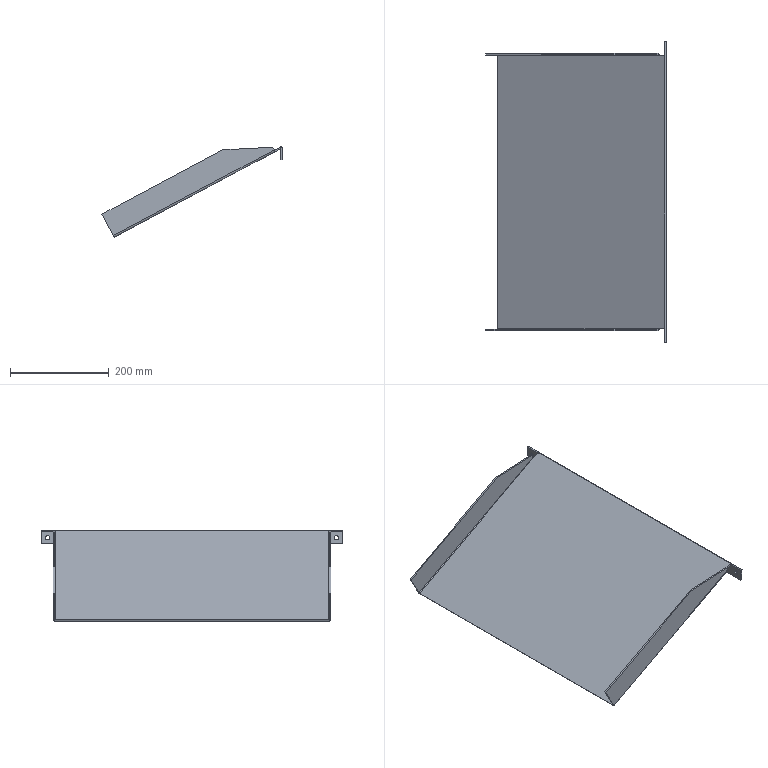Part | STEP file | lll_id3818_x_t | 1 solid | 27 faces | box 365.363 x 612 x 183.438 mm | volume 789228 mm3 | plane 20 | cylinder 7 | commonest cylinder face diameters 2 x2 8 x2 9 x2 3 x1
STEP:
#1=CARTESIAN_POINT('',(3904.435,-293.,-189.665));
#2=VERTEX_POINT('',#1);
#3=CARTESIAN_POINT('',(3904.435,-293.,-194.165));
#4=DIRECTION('',(1.,0.,0.));
#5=DIRECTION('',(0.,0.,1.));
#6=AXIS2_PLACEMENT_3D('',#3,#4,#5);
#7=CIRCLE('',#6,4.5);
#8=EDGE_CURVE('',#2,#2,#7,.T.);
#9=ORIENTED_EDGE('',*,*,#8,.T.);
#10=EDGE_LOOP('',(#9));
#11=FACE_BOUND('',#10,.T.);
#12=CARTESIAN_POINT('',(3904.435,293.,-189.665));
#13=VERTEX_POINT('',#12);
#14=CARTESIAN_POINT('',(3904.435,293.,-194.165));
#15=DIRECTION('',(1.,0.,0.));
#16=DIRECTION('',(0.,0.,1.));
#17=AXIS2_PLACEMENT_3D('',#14,#15,#16);
#18=CIRCLE('',#17,4.5);
#19=EDGE_CURVE('',#13,#13,#18,.T.);
#20=ORIENTED_EDGE('',*,*,#19,.T.);
#21=EDGE_LOOP('',(#20));
#22=FACE_BOUND('',#21,.T.);
#23=CARTESIAN_POINT('',(3904.435,276.,-181.5));
#24=VERTEX_POINT('',#23);
#25=CARTESIAN_POINT('',(3904.435,276.,-183.996));
#26=VERTEX_POINT('',#25);
#27=CARTESIAN_POINT('',(3904.435,276.,-170.446));
#28=DIRECTION('',(0.,0.,-1.));
#29=VECTOR('',#28,1.);
#30=LINE('',#27,#29);
#31=EDGE_CURVE('',#24,#26,#30,.T.);
#32=ORIENTED_EDGE('',*,*,#31,.F.);
#33=CARTESIAN_POINT('',(3904.435,306.,-181.5));
#34=VERTEX_POINT('',#33);
#35=CARTESIAN_POINT('',(3904.435,0.,-181.5));
#36=DIRECTION('',(0.,-1.,0.));
#37=VECTOR('',#36,1.);
#38=LINE('',#35,#37);
#39=EDGE_CURVE('',#34,#24,#38,.T.);
#40=ORIENTED_EDGE('',*,*,#39,.F.);
#41=CARTESIAN_POINT('',(3904.435,306.,-206.165));
#42=VERTEX_POINT('',#41);
#43=CARTESIAN_POINT('',(3904.435,306.,-170.446));
#44=DIRECTION('',(0.,0.,-1.));
#45=VECTOR('',#44,1.);
#46=LINE('',#43,#45);
#47=EDGE_CURVE('',#34,#42,#46,.T.);
#48=ORIENTED_EDGE('',*,*,#47,.T.);
#49=CARTESIAN_POINT('',(3904.435,-306.,-206.165));
#50=VERTEX_POINT('',#49);
#51=CARTESIAN_POINT('',(3904.435,110.,-206.165));
#52=DIRECTION('',(0.,-1.,0.));
#53=VECTOR('',#52,1.);
#54=LINE('',#51,#53);
#55=EDGE_CURVE('',#42,#50,#54,.T.);
#56=ORIENTED_EDGE('',*,*,#55,.T.);
#57=CARTESIAN_POINT('',(3904.435,-306.,-181.5));
#58=VERTEX_POINT('',#57);
#59=CARTESIAN_POINT('',(3904.435,-306.,-170.446));
#60=DIRECTION('',(0.,0.,1.));
#61=VECTOR('',#60,1.);
#62=LINE('',#59,#61);
#63=EDGE_CURVE('',#50,#58,#62,.T.);
#64=ORIENTED_EDGE('',*,*,#63,.T.);
#65=CARTESIAN_POINT('',(3904.435,-276.,-181.5));
#66=VERTEX_POINT('',#65);
#67=CARTESIAN_POINT('',(3904.435,0.,-181.5));
#68=DIRECTION('',(0.,-1.,0.));
#69=VECTOR('',#68,1.);
#70=LINE('',#67,#69);
#71=EDGE_CURVE('',#66,#58,#70,.T.);
#72=ORIENTED_EDGE('',*,*,#71,.F.);
#73=CARTESIAN_POINT('',(3904.435,-276.,-183.996));
#74=VERTEX_POINT('',#73);
#75=CARTESIAN_POINT('',(3904.435,-276.,-170.446));
#76=DIRECTION('',(0.,0.,1.));
#77=VECTOR('',#76,1.);
#78=LINE('',#75,#77);
#79=EDGE_CURVE('',#74,#66,#78,.T.);
#80=ORIENTED_EDGE('',*,*,#79,.F.);
#81=CARTESIAN_POINT('',(3904.435,110.,-183.996));
#82=DIRECTION('',(0.,-1.,0.));
#83=VECTOR('',#82,1.);
#84=LINE('',#81,#83);
#85=EDGE_CURVE('',#26,#74,#84,.T.);
#86=ORIENTED_EDGE('',*,*,#85,.F.);
#87=EDGE_LOOP('',(#32,#40,#48,#56,#64,#72,#80,#86));
#88=FACE_BOUND('',#87,.T.);
#89=CARTESIAN_POINT('',(3904.435,110.,-170.446));
#90=DIRECTION('',(1.,0.,0.));
#91=DIRECTION('',(0.,0.,-1.));
#92=AXIS2_PLACEMENT_3D('',#89,#90,#91);
#93=PLANE('',#92);
#94=ADVANCED_FACE('',(#11,#22,#88),#93,.F.);
#95=CARTESIAN_POINT('',(3907.435,-306.,-206.165));
#96=VERTEX_POINT('',#95);
#97=CARTESIAN_POINT('',(3907.435,-306.,-181.5));
#98=VERTEX_POINT('',#97);
#99=CARTESIAN_POINT('',(3907.435,-306.,-170.446));
#100=DIRECTION('',(0.,0.,1.));
#101=VECTOR('',#100,1.);
#102=LINE('',#99,#101);
#103=EDGE_CURVE('',#96,#98,#102,.T.);
#104=ORIENTED_EDGE('',*,*,#103,.F.);
#105=CARTESIAN_POINT('',(3907.435,306.,-206.165));
#106=VERTEX_POINT('',#105);
#107=CARTESIAN_POINT('',(3907.435,285.,-206.165));
#108=DIRECTION('',(0.,-1.,0.));
#109=VECTOR('',#108,1.);
#110=LINE('',#107,#109);
#111=EDGE_CURVE('',#106,#96,#110,.T.);
#112=ORIENTED_EDGE('',*,*,#111,.F.);
#113=CARTESIAN_POINT('',(3907.435,306.,-181.5));
#114=VERTEX_POINT('',#113);
#115=CARTESIAN_POINT('',(3907.435,306.,-170.446));
#116=DIRECTION('',(0.,0.,-1.));
#117=VECTOR('',#116,1.);
#118=LINE('',#115,#117);
#119=EDGE_CURVE('',#114,#106,#118,.T.);
#120=ORIENTED_EDGE('',*,*,#119,.F.);
#121=CARTESIAN_POINT('',(3907.435,36.,-181.5));
#122=DIRECTION('',(0.,1.,0.));
#123=VECTOR('',#122,1.);
#124=LINE('',#121,#123);
#125=EDGE_CURVE('',#98,#114,#124,.T.);
#126=ORIENTED_EDGE('',*,*,#125,.F.);
#127=EDGE_LOOP('',(#104,#112,#120,#126));
#128=FACE_BOUND('',#127,.T.);
#129=CARTESIAN_POINT('',(3907.435,293.,-198.665));
#130=VERTEX_POINT('',#129);
#131=CARTESIAN_POINT('',(3907.435,293.,-194.165));
#132=DIRECTION('',(1.,0.,0.));
#133=DIRECTION('',(0.,0.,-1.));
#134=AXIS2_PLACEMENT_3D('',#131,#132,#133);
#135=CIRCLE('',#134,4.5);
#136=EDGE_CURVE('',#130,#130,#135,.T.);
#137=ORIENTED_EDGE('',*,*,#136,.F.);
#138=EDGE_LOOP('',(#137));
#139=FACE_BOUND('',#138,.T.);
#140=CARTESIAN_POINT('',(3907.435,-293.,-198.665));
#141=VERTEX_POINT('',#140);
#142=CARTESIAN_POINT('',(3907.435,-293.,-194.165));
#143=DIRECTION('',(1.,0.,0.));
#144=DIRECTION('',(0.,0.,-1.));
#145=AXIS2_PLACEMENT_3D('',#142,#143,#144);
#146=CIRCLE('',#145,4.5);
#147=EDGE_CURVE('',#141,#141,#146,.T.);
#148=ORIENTED_EDGE('',*,*,#147,.F.);
#149=EDGE_LOOP('',(#148));
#150=FACE_BOUND('',#149,.T.);
#151=CARTESIAN_POINT('',(3907.435,110.,-170.446));
#152=DIRECTION('',(1.,0.,0.));
#153=DIRECTION('',(0.,0.,-1.));
#154=AXIS2_PLACEMENT_3D('',#151,#152,#153);
#155=PLANE('',#154);
#156=ADVANCED_FACE('',(#128,#139,#150),#155,.T.);
#157=ORIENTED_EDGE('',*,*,#103,.T.);
#158=CARTESIAN_POINT('',(3905.935,-306.,-181.5));
#159=DIRECTION('',(0.,1.,0.));
#160=DIRECTION('',(0.,0.,1.));
#161=AXIS2_PLACEMENT_3D('',#158,#159,#160);
#162=CIRCLE('',#161,1.5);
#163=EDGE_CURVE('',#58,#98,#162,.T.);
#164=ORIENTED_EDGE('',*,*,#163,.F.);
#165=ORIENTED_EDGE('',*,*,#63,.F.);
#166=CARTESIAN_POINT('',(3907.435,-306.,-206.165));
#167=DIRECTION('',(1.,0.,0.));
#168=VECTOR('',#167,1.);
#169=LINE('',#166,#168);
#170=EDGE_CURVE('',#50,#96,#169,.T.);
#171=ORIENTED_EDGE('',*,*,#170,.T.);
#172=EDGE_LOOP('',(#157,#164,#165,#171));
#173=FACE_OUTER_BOUND('',#172,.T.);
#174=CARTESIAN_POINT('',(3907.435,-306.,-173.053));
#175=DIRECTION('',(0.,1.,0.));
#176=DIRECTION('',(0.,0.,-1.));
#177=AXIS2_PLACEMENT_3D('',#174,#175,#176);
#178=PLANE('',#177);
#179=ADVANCED_FACE('',(#173),#178,.F.);
#180=ORIENTED_EDGE('',*,*,#170,.F.);
#181=ORIENTED_EDGE('',*,*,#55,.F.);
#182=CARTESIAN_POINT('',(3907.435,306.,-206.165));
#183=DIRECTION('',(1.,0.,0.));
#184=VECTOR('',#183,1.);
#185=LINE('',#182,#184);
#186=EDGE_CURVE('',#42,#106,#185,.T.);
#187=ORIENTED_EDGE('',*,*,#186,.T.);
#188=ORIENTED_EDGE('',*,*,#111,.T.);
#189=EDGE_LOOP('',(#180,#181,#187,#188));
#190=FACE_OUTER_BOUND('',#189,.T.);
#191=CARTESIAN_POINT('',(3907.435,285.,-206.165));
#192=DIRECTION('',(0.,0.,-1.));
#193=DIRECTION('',(0.,-1.,0.));
#194=AXIS2_PLACEMENT_3D('',#191,#192,#193);
#195=PLANE('',#194);
#196=ADVANCED_FACE('',(#190),#195,.T.);
#197=ORIENTED_EDGE('',*,*,#47,.F.);
#198=CARTESIAN_POINT('',(3905.935,306.,-181.5));
#199=DIRECTION('',(0.,-1.,0.));
#200=DIRECTION('',(1.,0.,0.));
#201=AXIS2_PLACEMENT_3D('',#198,#199,#200);
#202=CIRCLE('',#201,1.5);
#203=EDGE_CURVE('',#114,#34,#202,.T.);
#204=ORIENTED_EDGE('',*,*,#203,.F.);
#205=ORIENTED_EDGE('',*,*,#119,.T.);
#206=ORIENTED_EDGE('',*,*,#186,.F.);
#207=EDGE_LOOP('',(#197,#204,#205,#206));
#208=FACE_OUTER_BOUND('',#207,.T.);
#209=CARTESIAN_POINT('',(3887.906,306.,-180.316));
#210=DIRECTION('',(0.,-1.,0.));
#211=DIRECTION('',(-0.5,0.,0.866));
#212=AXIS2_PLACEMENT_3D('',#209,#210,#211);
#213=PLANE('',#212);
#214=ADVANCED_FACE('',(#208),#213,.F.);
#215=CARTESIAN_POINT('',(3891.925,276.,-187.25));
#216=VERTEX_POINT('',#215);
#217=CARTESIAN_POINT('',(3905.231,276.,-180.176));
#218=VERTEX_POINT('',#217);
#219=CARTESIAN_POINT('',(3906.063,276.,-179.733));
#220=DIRECTION('',(0.8829,0.,0.4695));
#221=VECTOR('',#220,1.);
#222=LINE('',#219,#221);
#223=EDGE_CURVE('',#216,#218,#222,.T.);
#224=ORIENTED_EDGE('',*,*,#223,.F.);
#225=CARTESIAN_POINT('',(3891.925,277.,-187.25));
#226=VERTEX_POINT('',#225);
#227=CARTESIAN_POINT('',(3891.925,-109.,-187.25));
#228=DIRECTION('',(0.,-1.,0.));
#229=VECTOR('',#228,1.);
#230=LINE('',#227,#229);
#231=EDGE_CURVE('',#226,#216,#230,.T.);
#232=ORIENTED_EDGE('',*,*,#231,.F.);
#233=CARTESIAN_POINT('',(3565.546,277.,-360.789));
#234=VERTEX_POINT('',#233);
#235=CARTESIAN_POINT('',(3985.528,277.,-137.481));
#236=DIRECTION('',(0.8829,0.,0.4695));
#237=VECTOR('',#236,1.);
#238=LINE('',#235,#237);
#239=EDGE_CURVE('',#234,#226,#238,.T.);
#240=ORIENTED_EDGE('',*,*,#239,.F.);
#241=CARTESIAN_POINT('',(3565.546,-277.,-360.789));
#242=VERTEX_POINT('',#241);
#243=CARTESIAN_POINT('',(3565.546,-35.,-360.789));
#244=DIRECTION('',(0.,1.,0.));
#245=VECTOR('',#244,1.);
#246=LINE('',#243,#245);
#247=EDGE_CURVE('',#242,#234,#246,.T.);
#248=ORIENTED_EDGE('',*,*,#247,.F.);
#249=CARTESIAN_POINT('',(3891.925,-277.,-187.25));
#250=VERTEX_POINT('',#249);
#251=CARTESIAN_POINT('',(3985.528,-277.,-137.481));
#252=DIRECTION('',(-0.8829,0.,-0.4695));
#253=VECTOR('',#252,1.);
#254=LINE('',#251,#253);
#255=EDGE_CURVE('',#250,#242,#254,.T.);
#256=ORIENTED_EDGE('',*,*,#255,.F.);
#257=CARTESIAN_POINT('',(3891.925,-276.,-187.25));
#258=VERTEX_POINT('',#257);
#259=CARTESIAN_POINT('',(3891.925,2.,-187.25));
#260=DIRECTION('',(0.,-1.,0.));
#261=VECTOR('',#260,1.);
#262=LINE('',#259,#261);
#263=EDGE_CURVE('',#258,#250,#262,.T.);
#264=ORIENTED_EDGE('',*,*,#263,.F.);
#265=CARTESIAN_POINT('',(3905.231,-276.,-180.176));
#266=VERTEX_POINT('',#265);
#267=CARTESIAN_POINT('',(3906.063,-276.,-179.733));
#268=DIRECTION('',(-0.8829,0.,-0.4695));
#269=VECTOR('',#268,1.);
#270=LINE('',#267,#269);
#271=EDGE_CURVE('',#266,#258,#270,.T.);
#272=ORIENTED_EDGE('',*,*,#271,.F.);
#273=CARTESIAN_POINT('',(3905.231,0.,-180.176));
#274=DIRECTION('',(0.,-1.,0.));
#275=VECTOR('',#274,1.);
#276=LINE('',#273,#275);
#277=EDGE_CURVE('',#218,#266,#276,.T.);
#278=ORIENTED_EDGE('',*,*,#277,.F.);
#279=EDGE_LOOP('',(#224,#232,#240,#248,#256,#264,#272,#278));
#280=FACE_OUTER_BOUND('',#279,.T.);
#281=CARTESIAN_POINT('',(3906.063,-35.,-179.733));
#282=DIRECTION('',(-0.4695,0.,0.8829));
#283=DIRECTION('',(-0.8829,0.,-0.4695));
#284=AXIS2_PLACEMENT_3D('',#281,#282,#283);
#285=PLANE('',#284);
#286=ADVANCED_FACE('',(#280),#285,.T.);
#287=CARTESIAN_POINT('',(3893.333,276.,-189.899));
#288=VERTEX_POINT('',#287);
#289=CARTESIAN_POINT('',(3891.925,276.,-187.25));
#290=DIRECTION('',(-0.4695,0.,0.8829));
#291=VECTOR('',#290,1.);
#292=LINE('',#289,#291);
#293=EDGE_CURVE('',#288,#216,#292,.T.);
#294=ORIENTED_EDGE('',*,*,#293,.T.);
#295=ORIENTED_EDGE('',*,*,#223,.T.);
#296=CARTESIAN_POINT('',(3905.935,276.,-181.5));
#297=DIRECTION('',(0.,1.,0.));
#298=DIRECTION('',(0.,0.,-1.));
#299=AXIS2_PLACEMENT_3D('',#296,#297,#298);
#300=CIRCLE('',#299,1.5);
#301=EDGE_CURVE('',#24,#218,#300,.T.);
#302=ORIENTED_EDGE('',*,*,#301,.F.);
#303=ORIENTED_EDGE('',*,*,#31,.T.);
#304=CARTESIAN_POINT('',(3907.471,276.,-182.382));
#305=DIRECTION('',(0.8829,0.,0.4695));
#306=VECTOR('',#305,1.);
#307=LINE('',#304,#306);
#308=EDGE_CURVE('',#288,#26,#307,.T.);
#309=ORIENTED_EDGE('',*,*,#308,.F.);
#310=EDGE_LOOP('',(#294,#295,#302,#303,#309));
#311=FACE_OUTER_BOUND('',#310,.T.);
#312=CARTESIAN_POINT('',(3906.155,276.,-179.742));
#313=DIRECTION('',(0.,-1.,0.));
#314=DIRECTION('',(-0.9063,0.,-0.4226));
#315=AXIS2_PLACEMENT_3D('',#312,#313,#314);
#316=PLANE('',#315);
#317=ADVANCED_FACE('',(#311),#316,.F.);
#318=ORIENTED_EDGE('',*,*,#271,.T.);
#319=CARTESIAN_POINT('',(3893.333,-276.,-189.899));
#320=VERTEX_POINT('',#319);
#321=CARTESIAN_POINT('',(3891.925,-276.,-187.25));
#322=DIRECTION('',(-0.4695,0.,0.8829));
#323=VECTOR('',#322,1.);
#324=LINE('',#321,#323);
#325=EDGE_CURVE('',#320,#258,#324,.T.);
#326=ORIENTED_EDGE('',*,*,#325,.F.);
#327=CARTESIAN_POINT('',(3907.471,-276.,-182.382));
#328=DIRECTION('',(-0.8829,0.,-0.4695));
#329=VECTOR('',#328,1.);
#330=LINE('',#327,#329);
#331=EDGE_CURVE('',#74,#320,#330,.T.);
#332=ORIENTED_EDGE('',*,*,#331,.F.);
#333=ORIENTED_EDGE('',*,*,#79,.T.);
#334=CARTESIAN_POINT('',(3905.935,-276.,-181.5));
#335=DIRECTION('',(0.,-1.,0.));
#336=DIRECTION('',(-1.,0.,0.));
#337=AXIS2_PLACEMENT_3D('',#334,#335,#336);
#338=CIRCLE('',#337,1.5);
#339=EDGE_CURVE('',#266,#66,#338,.T.);
#340=ORIENTED_EDGE('',*,*,#339,.F.);
#341=EDGE_LOOP('',(#318,#326,#332,#333,#340));
#342=FACE_OUTER_BOUND('',#341,.T.);
#343=CARTESIAN_POINT('',(3900.622,-276.,-159.655));
#344=DIRECTION('',(0.,1.,0.));
#345=DIRECTION('',(0.9962,0.,-0.08716));
#346=AXIS2_PLACEMENT_3D('',#343,#344,#345);
#347=PLANE('',#346);
#348=ADVANCED_FACE('',(#342),#347,.F.);
#349=ORIENTED_EDGE('',*,*,#163,.T.);
#350=ORIENTED_EDGE('',*,*,#125,.T.);
#351=ORIENTED_EDGE('',*,*,#203,.T.);
#352=ORIENTED_EDGE('',*,*,#39,.T.);
#353=ORIENTED_EDGE('',*,*,#301,.T.);
#354=ORIENTED_EDGE('',*,*,#277,.T.);
#355=ORIENTED_EDGE('',*,*,#339,.T.);
#356=ORIENTED_EDGE('',*,*,#71,.T.);
#357=EDGE_LOOP('',(#349,#350,#351,#352,#353,#354,#355,#356));
#358=FACE_OUTER_BOUND('',#357,.T.);
#359=CARTESIAN_POINT('',(3905.935,36.,-181.5));
#360=DIRECTION('',(0.,-1.,0.));
#361=DIRECTION('',(-0.9962,0.,0.08716));
#362=AXIS2_PLACEMENT_3D('',#359,#360,#361);
#363=CYLINDRICAL_SURFACE('',#362,1.5);
#364=ADVANCED_FACE('',(#358),#363,.T.);
#365=ORIENTED_EDGE('',*,*,#136,.T.);
#366=EDGE_LOOP('',(#365));
#367=FACE_BOUND('',#366,.T.);
#368=ORIENTED_EDGE('',*,*,#19,.F.);
#369=EDGE_LOOP('',(#368));
#370=FACE_BOUND('',#369,.T.);
#371=CARTESIAN_POINT('',(3907.435,293.,-194.165));
#372=DIRECTION('',(1.,0.,0.));
#373=DIRECTION('',(0.,-1.,0.));
#374=AXIS2_PLACEMENT_3D('',#371,#372,#373);
#375=CYLINDRICAL_SURFACE('',#374,4.5);
#376=ADVANCED_FACE('',(#367,#370),#375,.F.);
#377=ORIENTED_EDGE('',*,*,#147,.T.);
#378=EDGE_LOOP('',(#377));
#379=FACE_BOUND('',#378,.T.);
#380=ORIENTED_EDGE('',*,*,#8,.F.);
#381=EDGE_LOOP('',(#380));
#382=FACE_BOUND('',#381,.T.);
#383=CARTESIAN_POINT('',(3907.435,-293.,-194.165));
#384=DIRECTION('',(1.,0.,0.));
#385=DIRECTION('',(0.,-1.,0.));
#386=AXIS2_PLACEMENT_3D('',#383,#384,#385);
#387=CYLINDRICAL_SURFACE('',#386,4.5);
#388=ADVANCED_FACE('',(#379,#382),#387,.F.);
#389=ORIENTED_EDGE('',*,*,#308,.T.);
#390=ORIENTED_EDGE('',*,*,#85,.T.);
#391=ORIENTED_EDGE('',*,*,#331,.T.);
#392=CARTESIAN_POINT('',(3893.333,-277.,-189.899));
#393=VERTEX_POINT('',#392);
#394=CARTESIAN_POINT('',(3893.333,-35.,-189.899));
#395=DIRECTION('',(0.,-1.,0.));
#396=VECTOR('',#395,1.);
#397=LINE('',#394,#396);
#398=EDGE_CURVE('',#320,#393,#397,.T.);
#399=ORIENTED_EDGE('',*,*,#398,.T.);
#400=CARTESIAN_POINT('',(3566.954,-277.,-363.438));
#401=VERTEX_POINT('',#400);
#402=CARTESIAN_POINT('',(3986.937,-277.,-140.13));
#403=DIRECTION('',(-0.8829,0.,-0.4695));
#404=VECTOR('',#403,1.);
#405=LINE('',#402,#404);
#406=EDGE_CURVE('',#393,#401,#405,.T.);
#407=ORIENTED_EDGE('',*,*,#406,.T.);
#408=CARTESIAN_POINT('',(3566.954,277.,-363.438));
#409=VERTEX_POINT('',#408);
#410=CARTESIAN_POINT('',(3566.954,-35.,-363.438));
#411=DIRECTION('',(0.,1.,0.));
#412=VECTOR('',#411,1.);
#413=LINE('',#410,#412);
#414=EDGE_CURVE('',#401,#409,#413,.T.);
#415=ORIENTED_EDGE('',*,*,#414,.T.);
#416=CARTESIAN_POINT('',(3893.333,277.,-189.899));
#417=VERTEX_POINT('',#416);
#418=CARTESIAN_POINT('',(3986.937,277.,-140.13));
#419=DIRECTION('',(0.8829,0.,0.4695));
#420=VECTOR('',#419,1.);
#421=LINE('',#418,#420);
#422=EDGE_CURVE('',#409,#417,#421,.T.);
#423=ORIENTED_EDGE('',*,*,#422,.T.);
#424=CARTESIAN_POINT('',(3893.333,-35.,-189.899));
#425=DIRECTION('',(0.,-1.,0.));
#426=VECTOR('',#425,1.);
#427=LINE('',#424,#426);
#428=EDGE_CURVE('',#417,#288,#427,.T.);
#429=ORIENTED_EDGE('',*,*,#428,.T.);
#430=EDGE_LOOP('',(#389,#390,#391,#399,#407,#415,#423,#429));
#431=FACE_OUTER_BOUND('',#430,.T.);
#432=CARTESIAN_POINT('',(3907.471,-35.,-182.382));
#433=DIRECTION('',(-0.4695,0.,0.8829));
#434=DIRECTION('',(-0.8829,0.,-0.4695));
#435=AXIS2_PLACEMENT_3D('',#432,#433,#434);
#436=PLANE('',#435);
#437=ADVANCED_FACE('',(#431),#436,.F.);
#438=CARTESIAN_POINT('',(3787.377,-278.,-186.211));
#439=VERTEX_POINT('',#438);
#440=CARTESIAN_POINT('',(3787.377,-281.,-186.211));
#441=VERTEX_POINT('',#440);
#442=CARTESIAN_POINT('',(3787.377,-278.,-186.211));
#443=DIRECTION('',(0.,-1.,0.));
#444=VECTOR('',#443,1.);
#445=LINE('',#442,#444);
#446=EDGE_CURVE('',#439,#441,#445,.T.);
#447=ORIENTED_EDGE('',*,*,#446,.F.);
#448=CARTESIAN_POINT('',(3542.072,-278.,-316.642));
#449=VERTEX_POINT('',#448);
#450=CARTESIAN_POINT('',(3730.386,-278.,-216.514));
#451=DIRECTION('',(-0.8829,0.,-0.4695));
#452=VECTOR('',#451,1.);
#453=LINE('',#450,#452);
#454=EDGE_CURVE('',#439,#449,#453,.T.);
#455=ORIENTED_EDGE('',*,*,#454,.T.);
#456=CARTESIAN_POINT('',(3542.072,-281.,-316.642));
#457=VERTEX_POINT('',#456);
#458=CARTESIAN_POINT('',(3542.072,-278.,-316.642));
#459=DIRECTION('',(0.,-1.,0.));
#460=VECTOR('',#459,1.);
#461=LINE('',#458,#460);
#462=EDGE_CURVE('',#449,#457,#461,.T.);
#463=ORIENTED_EDGE('',*,*,#462,.T.);
#464=CARTESIAN_POINT('',(3730.386,-281.,-216.514));
#465=DIRECTION('',(-0.8829,0.,-0.4695));
#466=VECTOR('',#465,1.);
#467=LINE('',#464,#466);
#468=EDGE_CURVE('',#441,#457,#467,.T.);
#469=ORIENTED_EDGE('',*,*,#468,.F.);
#470=EDGE_LOOP('',(#447,#455,#463,#469));
#471=FACE_OUTER_BOUND('',#470,.T.);
#472=CARTESIAN_POINT('',(3730.386,-278.,-216.514));
#473=DIRECTION('',(0.4695,0.,-0.8829));
#474=DIRECTION('',(-0.8829,0.,-0.4695));
#475=AXIS2_PLACEMENT_3D('',#472,#473,#474);
#476=PLANE('',#475);
#477=ADVANCED_FACE('',(#471),#476,.F.);
#478=CARTESIAN_POINT('',(3888.553,-281.,-180.909));
#479=VERTEX_POINT('',#478);
#480=CARTESIAN_POINT('',(3888.553,-278.,-180.909));
#481=VERTEX_POINT('',#480);
#482=CARTESIAN_POINT('',(3888.553,-238.,-180.909));
#483=DIRECTION('',(0.,1.,0.));
#484=VECTOR('',#483,1.);
#485=LINE('',#482,#484);
#486=EDGE_CURVE('',#479,#481,#485,.T.);
#487=ORIENTED_EDGE('',*,*,#486,.F.);
#488=CARTESIAN_POINT('',(3891.456,-281.,-186.368));
#489=VERTEX_POINT('',#488);
#490=CARTESIAN_POINT('',(3891.925,-281.,-187.25));
#491=DIRECTION('',(-0.4695,0.,0.8829));
#492=VECTOR('',#491,1.);
#493=LINE('',#490,#492);
#494=EDGE_CURVE('',#489,#479,#493,.T.);
#495=ORIENTED_EDGE('',*,*,#494,.F.);
#496=CARTESIAN_POINT('',(3891.456,-277.,-186.368));
#497=DIRECTION('',(-0.8829,0.,-0.4695));
#498=DIRECTION('',(-0.4695,0.,0.8829));
#499=AXIS2_PLACEMENT_3D('',#496,#497,#498);
#500=CIRCLE('',#499,4.);
#501=EDGE_CURVE('',#393,#489,#500,.T.);
#502=ORIENTED_EDGE('',*,*,#501,.F.);
#503=ORIENTED_EDGE('',*,*,#398,.F.);
#504=ORIENTED_EDGE('',*,*,#325,.T.);
#505=ORIENTED_EDGE('',*,*,#263,.T.);
#506=CARTESIAN_POINT('',(3891.456,-278.,-186.368));
#507=VERTEX_POINT('',#506);
#508=CARTESIAN_POINT('',(3891.456,-277.,-186.368));
#509=DIRECTION('',(-0.8829,0.,-0.4695));
#510=DIRECTION('',(-0.4695,0.,0.8829));
#511=AXIS2_PLACEMENT_3D('',#508,#509,#510);
#512=CIRCLE('',#511,1.);
#513=EDGE_CURVE('',#250,#507,#512,.T.);
#514=ORIENTED_EDGE('',*,*,#513,.T.);
#515=CARTESIAN_POINT('',(3892.395,-278.,-188.133));
#516=DIRECTION('',(-0.4695,0.,0.8829));
#517=VECTOR('',#516,1.);
#518=LINE('',#515,#517);
#519=EDGE_CURVE('',#507,#481,#518,.T.);
#520=ORIENTED_EDGE('',*,*,#519,.T.);
#521=EDGE_LOOP('',(#487,#495,#502,#503,#504,#505,#514,#520));
#522=FACE_OUTER_BOUND('',#521,.T.);
#523=CARTESIAN_POINT('',(3891.925,-238.,-187.25));
#524=DIRECTION('',(0.8829,0.,0.4695));
#525=DIRECTION('',(0.,-1.,0.));
#526=AXIS2_PLACEMENT_3D('',#523,#524,#525);
#527=PLANE('',#526);
#528=ADVANCED_FACE('',(#522),#527,.T.);
#529=CARTESIAN_POINT('',(3888.553,281.,-180.909));
#530=VERTEX_POINT('',#529);
#531=CARTESIAN_POINT('',(3888.553,278.,-180.909));
#532=VERTEX_POINT('',#531);
#533=CARTESIAN_POINT('',(3888.553,278.,-180.909));
#534=DIRECTION('',(0.,-1.,0.));
#535=VECTOR('',#534,1.);
#536=LINE('',#533,#535);
#537=EDGE_CURVE('',#530,#532,#536,.T.);
#538=ORIENTED_EDGE('',*,*,#537,.T.);
#539=CARTESIAN_POINT('',(3891.456,278.,-186.368));
#540=VERTEX_POINT('',#539);
#541=CARTESIAN_POINT('',(3891.456,278.,-186.368));
#542=DIRECTION('',(0.4695,0.,-0.8829));
#543=VECTOR('',#542,1.);
#544=LINE('',#541,#543);
#545=EDGE_CURVE('',#532,#540,#544,.T.);
#546=ORIENTED_EDGE('',*,*,#545,.T.);
#547=CARTESIAN_POINT('',(3891.456,277.,-186.368));
#548=DIRECTION('',(-0.8829,0.,-0.4695));
#549=DIRECTION('',(-0.4695,0.,0.8829));
#550=AXIS2_PLACEMENT_3D('',#547,#548,#549);
#551=CIRCLE('',#550,1.);
#552=EDGE_CURVE('',#540,#226,#551,.T.);
#553=ORIENTED_EDGE('',*,*,#552,.T.);
#554=ORIENTED_EDGE('',*,*,#231,.T.);
#555=ORIENTED_EDGE('',*,*,#293,.F.);
#556=ORIENTED_EDGE('',*,*,#428,.F.);
#557=CARTESIAN_POINT('',(3891.456,281.,-186.368));
#558=VERTEX_POINT('',#557);
#559=CARTESIAN_POINT('',(3891.456,277.,-186.368));
#560=DIRECTION('',(-0.8829,0.,-0.4695));
#561=DIRECTION('',(-0.4695,0.,0.8829));
#562=AXIS2_PLACEMENT_3D('',#559,#560,#561);
#563=CIRCLE('',#562,4.);
#564=EDGE_CURVE('',#558,#417,#563,.T.);
#565=ORIENTED_EDGE('',*,*,#564,.F.);
#566=CARTESIAN_POINT('',(3891.456,281.,-186.368));
#567=DIRECTION('',(0.4695,0.,-0.8829));
#568=VECTOR('',#567,1.);
#569=LINE('',#566,#568);
#570=EDGE_CURVE('',#530,#558,#569,.T.);
#571=ORIENTED_EDGE('',*,*,#570,.F.);
#572=EDGE_LOOP('',(#538,#546,#553,#554,#555,#556,#565,#571));
#573=FACE_OUTER_BOUND('',#572,.T.);
#574=CARTESIAN_POINT('',(3891.456,278.,-186.368));
#575=DIRECTION('',(0.8829,0.,0.4695));
#576=DIRECTION('',(-0.4695,0.,0.8829));
#577=AXIS2_PLACEMENT_3D('',#574,#575,#576);
#578=PLANE('',#577);
#579=ADVANCED_FACE('',(#573),#578,.T.);
#580=CARTESIAN_POINT('',(3787.377,281.,-186.211));
#581=VERTEX_POINT('',#580);
#582=CARTESIAN_POINT('',(3787.377,278.,-186.211));
#583=VERTEX_POINT('',#582);
#584=CARTESIAN_POINT('',(3787.377,278.,-186.211));
#585=DIRECTION('',(0.,-1.,0.));
#586=VECTOR('',#585,1.);
#587=LINE('',#584,#586);
#588=EDGE_CURVE('',#581,#583,#587,.T.);
#589=ORIENTED_EDGE('',*,*,#588,.F.);
#590=CARTESIAN_POINT('',(3542.072,281.,-316.642));
#591=VERTEX_POINT('',#590);
#592=CARTESIAN_POINT('',(3730.386,281.,-216.514));
#593=DIRECTION('',(0.8829,0.,0.4695));
#594=VECTOR('',#593,1.);
#595=LINE('',#592,#594);
#596=EDGE_CURVE('',#591,#581,#595,.T.);
#597=ORIENTED_EDGE('',*,*,#596,.F.);
#598=CARTESIAN_POINT('',(3542.072,278.,-316.642));
#599=VERTEX_POINT('',#598);
#600=CARTESIAN_POINT('',(3542.072,-35.,-316.642));
#601=DIRECTION('',(0.,1.,0.));
#602=VECTOR('',#601,1.);
#603=LINE('',#600,#602);
#604=EDGE_CURVE('',#599,#591,#603,.T.);
#605=ORIENTED_EDGE('',*,*,#604,.F.);
#606=CARTESIAN_POINT('',(3730.386,278.,-216.514));
#607=DIRECTION('',(0.8829,0.,0.4695));
#608=VECTOR('',#607,1.);
#609=LINE('',#606,#608);
#610=EDGE_CURVE('',#599,#583,#609,.T.);
#611=ORIENTED_EDGE('',*,*,#610,.T.);
#612=EDGE_LOOP('',(#589,#597,#605,#611));
#613=FACE_OUTER_BOUND('',#612,.T.);
#614=CARTESIAN_POINT('',(3730.386,278.,-216.514));
#615=DIRECTION('',(0.4695,0.,-0.8829));
#616=DIRECTION('',(0.8829,0.,0.4695));
#617=AXIS2_PLACEMENT_3D('',#614,#615,#616);
#618=PLANE('',#617);
#619=ADVANCED_FACE('',(#613),#618,.F.);
#620=CARTESIAN_POINT('',(3987.162,-278.,-175.741));
#621=DIRECTION('',(-0.9986,0.,-0.05234));
#622=VECTOR('',#621,1.);
#623=LINE('',#620,#622);
#624=EDGE_CURVE('',#481,#439,#623,.T.);
#625=ORIENTED_EDGE('',*,*,#624,.F.);
#626=ORIENTED_EDGE('',*,*,#519,.F.);
#627=CARTESIAN_POINT('',(3565.077,-278.,-359.906));
#628=VERTEX_POINT('',#627);
#629=CARTESIAN_POINT('',(3984.286,-278.,-137.009));
#630=DIRECTION('',(0.8829,0.,0.4695));
#631=VECTOR('',#630,1.);
#632=LINE('',#629,#631);
#633=EDGE_CURVE('',#628,#507,#632,.T.);
#634=ORIENTED_EDGE('',*,*,#633,.F.);
#635=CARTESIAN_POINT('',(3565.546,-278.,-360.789));
#636=DIRECTION('',(0.4695,0.,-0.8829));
#637=VECTOR('',#636,1.);
#638=LINE('',#635,#637);
#639=EDGE_CURVE('',#449,#628,#638,.T.);
#640=ORIENTED_EDGE('',*,*,#639,.F.);
#641=ORIENTED_EDGE('',*,*,#454,.F.);
#642=EDGE_LOOP('',(#625,#626,#634,#640,#641));
#643=FACE_OUTER_BOUND('',#642,.T.);
#644=CARTESIAN_POINT('',(3985.225,-278.,-138.775));
#645=DIRECTION('',(0.,-1.,0.));
#646=DIRECTION('',(-0.2924,0.,-0.9563));
#647=AXIS2_PLACEMENT_3D('',#644,#645,#646);
#648=PLANE('',#647);
#649=ADVANCED_FACE('',(#643),#648,.F.);
#650=CARTESIAN_POINT('',(3986.888,278.,-175.755));
#651=DIRECTION('',(-0.9986,0.,-0.05234));
#652=VECTOR('',#651,1.);
#653=LINE('',#650,#652);
#654=EDGE_CURVE('',#532,#583,#653,.T.);
#655=ORIENTED_EDGE('',*,*,#654,.T.);
#656=ORIENTED_EDGE('',*,*,#610,.F.);
#657=CARTESIAN_POINT('',(3565.077,278.,-359.906));
#658=VERTEX_POINT('',#657);
#659=CARTESIAN_POINT('',(3565.546,278.,-360.789));
#660=DIRECTION('',(-0.4695,0.,0.8829));
#661=VECTOR('',#660,1.);
#662=LINE('',#659,#661);
#663=EDGE_CURVE('',#658,#599,#662,.T.);
#664=ORIENTED_EDGE('',*,*,#663,.F.);
#665=CARTESIAN_POINT('',(3984.103,278.,-137.106));
#666=DIRECTION('',(-0.8829,0.,-0.4695));
#667=VECTOR('',#666,1.);
#668=LINE('',#665,#667);
#669=EDGE_CURVE('',#540,#658,#668,.T.);
#670=ORIENTED_EDGE('',*,*,#669,.F.);
#671=ORIENTED_EDGE('',*,*,#545,.F.);
#672=EDGE_LOOP('',(#655,#656,#664,#670,#671));
#673=FACE_OUTER_BOUND('',#672,.T.);
#674=CARTESIAN_POINT('',(3984.945,278.,-138.689));
#675=DIRECTION('',(0.,1.,0.));
#676=DIRECTION('',(0.2924,0.,0.9563));
#677=AXIS2_PLACEMENT_3D('',#674,#675,#676);
#678=PLANE('',#677);
#679=ADVANCED_FACE('',(#673),#678,.F.);
#680=ORIENTED_EDGE('',*,*,#494,.T.);
#681=CARTESIAN_POINT('',(3987.162,-281.,-175.741));
#682=DIRECTION('',(-0.9986,0.,-0.05234));
#683=VECTOR('',#682,1.);
#684=LINE('',#681,#683);
#685=EDGE_CURVE('',#479,#441,#684,.T.);
#686=ORIENTED_EDGE('',*,*,#685,.T.);
#687=ORIENTED_EDGE('',*,*,#468,.T.);
#688=CARTESIAN_POINT('',(3565.077,-281.,-359.906));
#689=VERTEX_POINT('',#688);
#690=CARTESIAN_POINT('',(3565.546,-281.,-360.789));
#691=DIRECTION('',(0.4695,0.,-0.8829));
#692=VECTOR('',#691,1.);
#693=LINE('',#690,#692);
#694=EDGE_CURVE('',#457,#689,#693,.T.);
#695=ORIENTED_EDGE('',*,*,#694,.T.);
#696=CARTESIAN_POINT('',(3985.059,-281.,-136.598));
#697=DIRECTION('',(0.8829,0.,0.4695));
#698=VECTOR('',#697,1.);
#699=LINE('',#696,#698);
#700=EDGE_CURVE('',#689,#489,#699,.T.);
#701=ORIENTED_EDGE('',*,*,#700,.T.);
#702=EDGE_LOOP('',(#680,#686,#687,#695,#701));
#703=FACE_OUTER_BOUND('',#702,.T.);
#704=CARTESIAN_POINT('',(3985.225,-281.,-138.775));
#705=DIRECTION('',(0.,-1.,0.));
#706=DIRECTION('',(-0.2924,0.,-0.9563));
#707=AXIS2_PLACEMENT_3D('',#704,#705,#706);
#708=PLANE('',#707);
#709=ADVANCED_FACE('',(#703),#708,.T.);
#710=ORIENTED_EDGE('',*,*,#596,.T.);
#711=CARTESIAN_POINT('',(3986.888,281.,-175.755));
#712=DIRECTION('',(0.9986,0.,0.05234));
#713=VECTOR('',#712,1.);
#714=LINE('',#711,#713);
#715=EDGE_CURVE('',#581,#530,#714,.T.);
#716=ORIENTED_EDGE('',*,*,#715,.T.);
#717=ORIENTED_EDGE('',*,*,#570,.T.);
#718=CARTESIAN_POINT('',(3565.077,281.,-359.906));
#719=VERTEX_POINT('',#718);
#720=CARTESIAN_POINT('',(3985.059,281.,-136.598));
#721=DIRECTION('',(-0.8829,0.,-0.4695));
#722=VECTOR('',#721,1.);
#723=LINE('',#720,#722);
#724=EDGE_CURVE('',#558,#719,#723,.T.);
#725=ORIENTED_EDGE('',*,*,#724,.T.);
#726=CARTESIAN_POINT('',(3565.546,281.,-360.789));
#727=DIRECTION('',(-0.4695,0.,0.8829));
#728=VECTOR('',#727,1.);
#729=LINE('',#726,#728);
#730=EDGE_CURVE('',#719,#591,#729,.T.);
#731=ORIENTED_EDGE('',*,*,#730,.T.);
#732=EDGE_LOOP('',(#710,#716,#717,#725,#731));
#733=FACE_OUTER_BOUND('',#732,.T.);
#734=CARTESIAN_POINT('',(3984.945,281.,-138.689));
#735=DIRECTION('',(0.,1.,0.));
#736=DIRECTION('',(0.2924,0.,0.9563));
#737=AXIS2_PLACEMENT_3D('',#734,#735,#736);
#738=PLANE('',#737);
#739=ADVANCED_FACE('',(#733),#738,.T.);
#740=ORIENTED_EDGE('',*,*,#414,.F.);
#741=CARTESIAN_POINT('',(3565.077,-277.,-359.906));
#742=DIRECTION('',(0.8829,0.,0.4695));
#743=DIRECTION('',(0.4695,0.,-0.8829));
#744=AXIS2_PLACEMENT_3D('',#741,#742,#743);
#745=CIRCLE('',#744,4.);
#746=EDGE_CURVE('',#689,#401,#745,.T.);
#747=ORIENTED_EDGE('',*,*,#746,.F.);
#748=ORIENTED_EDGE('',*,*,#694,.F.);
#749=ORIENTED_EDGE('',*,*,#462,.F.);
#750=ORIENTED_EDGE('',*,*,#639,.T.);
#751=CARTESIAN_POINT('',(3565.077,-277.,-359.906));
#752=DIRECTION('',(0.8829,0.,0.4695));
#753=DIRECTION('',(0.4695,0.,-0.8829));
#754=AXIS2_PLACEMENT_3D('',#751,#752,#753);
#755=CIRCLE('',#754,1.);
#756=EDGE_CURVE('',#628,#242,#755,.T.);
#757=ORIENTED_EDGE('',*,*,#756,.T.);
#758=ORIENTED_EDGE('',*,*,#247,.T.);
#759=CARTESIAN_POINT('',(3565.077,277.,-359.906));
#760=DIRECTION('',(0.8829,0.,0.4695));
#761=DIRECTION('',(0.4695,0.,-0.8829));
#762=AXIS2_PLACEMENT_3D('',#759,#760,#761);
#763=CIRCLE('',#762,1.);
#764=EDGE_CURVE('',#234,#658,#763,.T.);
#765=ORIENTED_EDGE('',*,*,#764,.T.);
#766=ORIENTED_EDGE('',*,*,#663,.T.);
#767=ORIENTED_EDGE('',*,*,#604,.T.);
#768=ORIENTED_EDGE('',*,*,#730,.F.);
#769=CARTESIAN_POINT('',(3565.077,277.,-359.906));
#770=DIRECTION('',(0.8829,0.,0.4695));
#771=DIRECTION('',(0.4695,0.,-0.8829));
#772=AXIS2_PLACEMENT_3D('',#769,#770,#771);
#773=CIRCLE('',#772,4.);
#774=EDGE_CURVE('',#409,#719,#773,.T.);
#775=ORIENTED_EDGE('',*,*,#774,.F.);
#776=EDGE_LOOP('',(#740,#747,#748,#749,#750,#757,#758,#765,#766,#767,#768,#775));
#777=FACE_OUTER_BOUND('',#776,.T.);
#778=CARTESIAN_POINT('',(3565.546,-35.,-360.789));
#779=DIRECTION('',(0.8829,0.,0.4695));
#780=DIRECTION('',(0.,-1.,0.));
#781=AXIS2_PLACEMENT_3D('',#778,#779,#780);
#782=PLANE('',#781);
#783=ADVANCED_FACE('',(#777),#782,.F.);
#784=ORIENTED_EDGE('',*,*,#669,.T.);
#785=ORIENTED_EDGE('',*,*,#764,.F.);
#786=ORIENTED_EDGE('',*,*,#239,.T.);
#787=ORIENTED_EDGE('',*,*,#552,.F.);
#788=EDGE_LOOP('',(#784,#785,#786,#787));
#789=FACE_OUTER_BOUND('',#788,.T.);
#790=CARTESIAN_POINT('',(3985.059,277.,-136.598));
#791=DIRECTION('',(0.8829,0.,0.4695));
#792=DIRECTION('',(-0.4695,0.,0.8829));
#793=AXIS2_PLACEMENT_3D('',#790,#791,#792);
#794=CYLINDRICAL_SURFACE('',#793,1.);
#795=ADVANCED_FACE('',(#789),#794,.F.);
#796=ORIENTED_EDGE('',*,*,#255,.T.);
#797=ORIENTED_EDGE('',*,*,#756,.F.);
#798=ORIENTED_EDGE('',*,*,#633,.T.);
#799=ORIENTED_EDGE('',*,*,#513,.F.);
#800=EDGE_LOOP('',(#796,#797,#798,#799));
#801=FACE_OUTER_BOUND('',#800,.T.);
#802=CARTESIAN_POINT('',(3985.059,-277.,-136.598));
#803=DIRECTION('',(-0.8829,0.,-0.4695));
#804=DIRECTION('',(0.4695,0.,-0.8829));
#805=AXIS2_PLACEMENT_3D('',#802,#803,#804);
#806=CYLINDRICAL_SURFACE('',#805,1.);
#807=ADVANCED_FACE('',(#801),#806,.F.);
#808=ORIENTED_EDGE('',*,*,#724,.F.);
#809=ORIENTED_EDGE('',*,*,#564,.T.);
#810=ORIENTED_EDGE('',*,*,#422,.F.);
#811=ORIENTED_EDGE('',*,*,#774,.T.);
#812=EDGE_LOOP('',(#808,#809,#810,#811));
#813=FACE_OUTER_BOUND('',#812,.T.);
#814=CARTESIAN_POINT('',(3985.059,277.,-136.598));
#815=DIRECTION('',(0.8829,0.,0.4695));
#816=DIRECTION('',(-0.4695,0.,0.8829));
#817=AXIS2_PLACEMENT_3D('',#814,#815,#816);
#818=CYLINDRICAL_SURFACE('',#817,4.);
#819=ADVANCED_FACE('',(#813),#818,.T.);
#820=ORIENTED_EDGE('',*,*,#406,.F.);
#821=ORIENTED_EDGE('',*,*,#501,.T.);
#822=ORIENTED_EDGE('',*,*,#700,.F.);
#823=ORIENTED_EDGE('',*,*,#746,.T.);
#824=EDGE_LOOP('',(#820,#821,#822,#823));
#825=FACE_OUTER_BOUND('',#824,.T.);
#826=CARTESIAN_POINT('',(3985.059,-277.,-136.598));
#827=DIRECTION('',(-0.8829,0.,-0.4695));
#828=DIRECTION('',(0.4695,0.,-0.8829));
#829=AXIS2_PLACEMENT_3D('',#826,#827,#828);
#830=CYLINDRICAL_SURFACE('',#829,4.);
#831=ADVANCED_FACE('',(#825),#830,.T.);
#832=ORIENTED_EDGE('',*,*,#588,.T.);
#833=ORIENTED_EDGE('',*,*,#654,.F.);
#834=ORIENTED_EDGE('',*,*,#537,.F.);
#835=ORIENTED_EDGE('',*,*,#715,.F.);
#836=EDGE_LOOP('',(#832,#833,#834,#835));
#837=FACE_OUTER_BOUND('',#836,.T.);
#838=CARTESIAN_POINT('',(3937.314,0.,-178.353));
#839=DIRECTION('',(-0.05234,0.,0.9986));
#840=DIRECTION('',(0.9986,0.,0.05234));
#841=AXIS2_PLACEMENT_3D('',#838,#839,#840);
#842=PLANE('',#841);
#843=ADVANCED_FACE('',(#837),#842,.T.);
#844=ORIENTED_EDGE('',*,*,#486,.T.);
#845=ORIENTED_EDGE('',*,*,#624,.T.);
#846=ORIENTED_EDGE('',*,*,#446,.T.);
#847=ORIENTED_EDGE('',*,*,#685,.F.);
#848=EDGE_LOOP('',(#844,#845,#846,#847));
#849=FACE_OUTER_BOUND('',#848,.T.);
#850=CARTESIAN_POINT('',(3937.314,0.,-178.353));
#851=DIRECTION('',(-0.05234,0.,0.9986));
#852=DIRECTION('',(0.9986,0.,0.05234));
#853=AXIS2_PLACEMENT_3D('',#850,#851,#852);
#854=PLANE('',#853);
#855=ADVANCED_FACE('',(#849),#854,.T.);
#856=CLOSED_SHELL('',(#94,#156,#179,#196,#214,#286,#317,#348,#364,#376,#388,#437,#477,#528,#579,#619,#649,#679,#709,#739,#783,#795,#807,#819,#831,#843,#855));
#857=MANIFOLD_SOLID_BREP('',#856);
#858=(LENGTH_UNIT()NAMED_UNIT(*)SI_UNIT(.MILLI.,.METRE.));
#859=UNCERTAINTY_MEASURE_WITH_UNIT(LENGTH_MEASURE(0.00002),#858,'','');
#860=(NAMED_UNIT(*)PLANE_ANGLE_UNIT()SI_UNIT($,.RADIAN.));
#861=PLANE_ANGLE_MEASURE_WITH_UNIT(PLANE_ANGLE_MEASURE(0.01745),#860);
#862=DIMENSIONAL_EXPONENTS(0.,0.,0.,0.,0.,0.,0.);
#863=(CONVERSION_BASED_UNIT('DEGREE',#861)NAMED_UNIT(#862)PLANE_ANGLE_UNIT());
#864=(NAMED_UNIT(*)SI_UNIT($,.STERADIAN.)SOLID_ANGLE_UNIT());
#865=(GEOMETRIC_REPRESENTATION_CONTEXT(3)GLOBAL_UNCERTAINTY_ASSIGNED_CONTEXT((#859))GLOBAL_UNIT_ASSIGNED_CONTEXT((#858,#863,#864))REPRESENTATION_CONTEXT('',''));
#866=ADVANCED_BREP_SHAPE_REPRESENTATION('',(#857),#865);